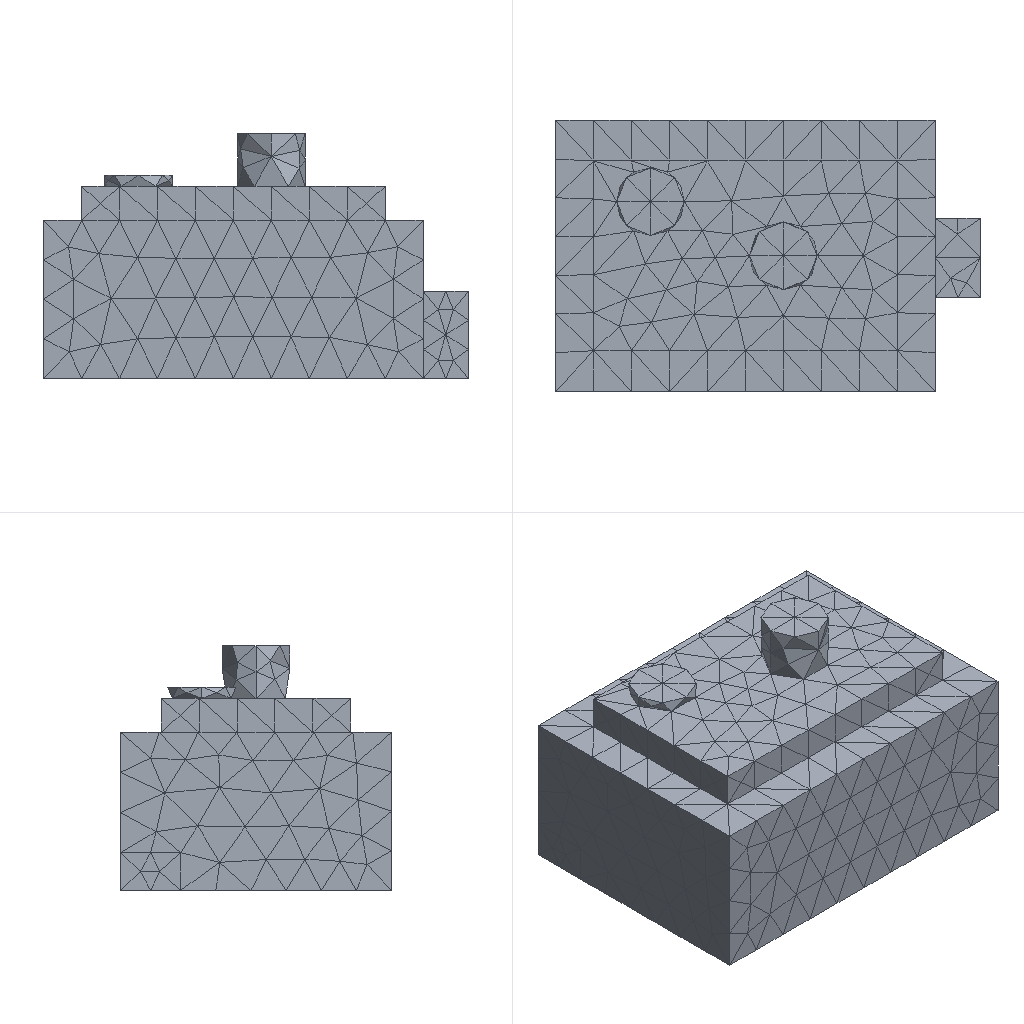Simulation study | ansys mapdl
Set-up summary:
category,name,step,type,value,unit,region
solver,ansys_mapdl
units,mm-N-s-tonne (MPa),,inferred,E=210000 density=
analysis,model,,static
mesh,nodes,,,4727
mesh,elements,,,2837
element_type,SOLID187,,,2837
material,mat 1,,E,210000
material,mat 1,,nu,0.3
load,,model,body load temp,,,all
load,,model,force,"1000 [dir=(0, 0, -1) n=169]",,node list
bc,,model,fixed,"[dofs=UX,UY,UZ n=5242]",,node list
Ansys APDL input file, long lists of numbers shortened:
/COM,ANSYS RELEASE 2026 R1           BUILD 26.1      UP20260202       09:09:40
/PREP7
/NOPR
/TITLE,2
ANTYPE, 0
*IF,_CDRDOFF,EQ,1,THEN     !if solid model was read in
_CDRDOFF=             !reset flag, numoffs already performed
*ELSE              !offset database for the following FE model
NUMOFF,NODE,     4727
NUMOFF,ELEM,     2837
NUMOFF,MAT ,        1
NUMOFF,TYPE,        1
*ENDIF
*SET,_RETURN ,  0.
*SET,_STATUS ,  0.
*SET,_UIQR   ,  169.
*SET,__FLOATPARAMETER__,  4727.
DOF,DELETE
ETBLOCK,        1,        1
(2i9,19a9)
        1      187        0        0        0        0        0        0        0        0        0        0        0        0        0        0        0        0        0        0        0
       -1
NBLOCK,6,SOLID,      4727,      4727
(3i9,6e21.13e3)
        1        0        0-3.4425000000000E+001 3.6000000000000E+001 1.0000000000000E+001
! (4726 more lines like these left out)
N,UNBL,LOC,       -1,
EBLOCK,19,SOLID,      2837,      2837
(19i10)
         1         1         1         1         0         0         0         0        10         0         1      1791      1792      1793      1794      2064      2065      2066      2067
! (5673 more lines like these left out)
        -1
MPTEMP,UNBL, 1, 1,  0.    ,
MPDATA,UNBL, 1,EX  ,       1, 1,  210000.000    ,
MPTEMP,UNBL, 1, 1,  0.    ,
MPDATA,UNBL, 1,NUXY,       1, 1, 0.3    ,
MPTEMP,UNBL, 1, 1,  0.    ,
MPDATA,UNBL, 1,PRXY,       1, 1, 0.3    ,
EXTOPT,ATTR,      0,      0,      0
EXTOPT,ESIZE,  0,  0.
EXTOPT,ACLEAR,      0
TREF,  0.
IRLF,  0
BFUNIF,TEMP,_TINY
ACEL,  0.    ,  0.    ,  0.
OMEGA,  0.    ,  0.    ,  0.
DOMEGA,  0.    ,  0.    ,  0.
CGLOC,  0.    ,  0.    ,  0.
CGOMEGA,  0.    ,  0.    ,  0.
DCGOMG,  0.    ,  0.    ,  0.
KUSE,     0
TIME,  0.
ALPHAD,  0.
BETAD,  0.
DMPRAT,  0.
DMPSTR,  0.
CRPLIM, 0.1    ,   0
CRPLIM,  0.    ,   1
NCNV,     0, 1.000000000E+12,     0,  0.    ,  0.
NEQIT,     0
ERESX,DEFA
DBLOCK,      5242
(i9,a6,2(pg16.9))
        1  UX    0.00000000      0.00000000
! (5241 more lines like these left out)
       -1
FBLOCK,       169
(i9,a6,2(pg16.9))
      828  FZ   -5.91715976      0.00000000
! (168 more lines like these left out)
       -1
/GO
FINISH
Results summary:
result,analysis_type_db,,,static,unstated
result,n_sets,,,1,unstated
result,load_steps[0].set,load_step=1,,1,unstated
result,load_steps[0].substep,load_step=1,,1,unstated
result,load_steps[0].time,load_step=1,,1,unstated
result,load_steps[0].freq,load_step=1,,1,unstated
result,load_steps[0].max_usum,load_step=1,,0.0003391,unstated
result,load_steps[0].max_seqv,load_step=1,,3.141,unstated
result,load_steps[0].reaction_sum.FX,load_step=1,,-8.44785e-12,unstated
result,load_steps[0].reaction_sum.FY,load_step=1,,-7.74891e-12,unstated
result,load_steps[0].reaction_sum.FZ,load_step=1,,1000,unstated
result,load_steps[0].reaction_sum.MX,load_step=1,,0,unstated
result,load_steps[0].reaction_sum.MY,load_step=1,,0,unstated
result,load_steps[0].reaction_sum.MZ,load_step=1,,0,unstated
result,convergence,,,results present for all listed sets,unstated